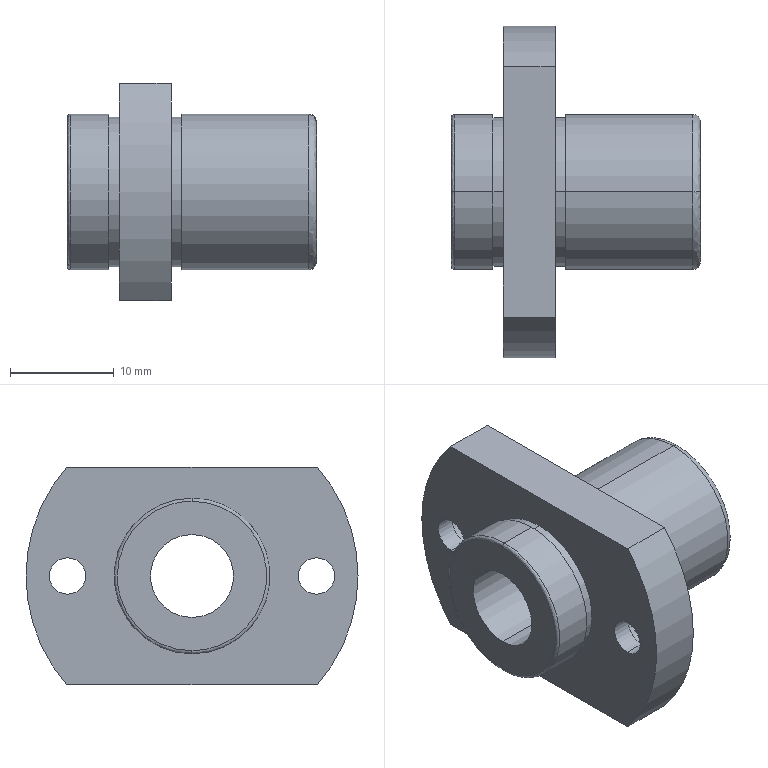Part | STEP file | LHIFC-N8 | 1 solid | 34 faces | box 24 x 32 x 21 mm | volume 5005 mm3 | cylinder 20 | plane 10 | spline 4 | commonest cylinder face diameters 3.5 x4 6 x4 14.4 x4 15 x4 8 x2 32 x2
STEP:
#1=CARTESIAN_POINT('',(0.,0.,7.2));
#2=VERTEX_POINT('',#1);
#3=CARTESIAN_POINT('',(0.,0.,-7.2));
#4=VERTEX_POINT('',#3);
#5=CARTESIAN_POINT('',(0.,0.,7.2));
#6=CARTESIAN_POINT('',(0.,-14.4,7.2));
#7=CARTESIAN_POINT('',(0.,-14.4,-7.2));
#8=CARTESIAN_POINT('',(0.,0.,-7.2));
#9=(BOUNDED_CURVE()B_SPLINE_CURVE(3,(#5,#6,#7,#8),.UNSPECIFIED.,.F.,.F.)B_SPLINE_CURVE_WITH_KNOTS((4,4),(0.,1.),.UNSPECIFIED.)CURVE()GEOMETRIC_REPRESENTATION_ITEM()RATIONAL_B_SPLINE_CURVE((1.,0.3333,0.3333,1.))REPRESENTATION_ITEM(''));
#10=EDGE_CURVE('',#2,#4,#9,.T.);
#11=ORIENTED_EDGE('',*,*,#10,.T.);
#12=CARTESIAN_POINT('',(0.3,0.,-7.5));
#13=VERTEX_POINT('',#12);
#14=CARTESIAN_POINT('',(0.3,0.,-7.2));
#15=DIRECTION('',(0.,-1.,0.));
#16=DIRECTION('',(0.,0.,-1.));
#17=AXIS2_PLACEMENT_3D('',#14,#15,#16);
#18=CIRCLE('',#17,0.3);
#19=EDGE_CURVE('',#4,#13,#18,.T.);
#20=ORIENTED_EDGE('',*,*,#19,.T.);
#21=CARTESIAN_POINT('',(0.3,0.,7.5));
#22=VERTEX_POINT('',#21);
#23=CARTESIAN_POINT('',(0.3,0.,0.));
#24=DIRECTION('',(1.,0.,0.));
#25=DIRECTION('',(0.,0.,-1.));
#26=AXIS2_PLACEMENT_3D('',#23,#24,#25);
#27=CIRCLE('',#26,7.5);
#28=EDGE_CURVE('',#22,#13,#27,.T.);
#29=ORIENTED_EDGE('',*,*,#28,.F.);
#30=CARTESIAN_POINT('',(0.3,0.,7.2));
#31=DIRECTION('',(0.,1.,0.));
#32=DIRECTION('',(0.,0.,1.));
#33=AXIS2_PLACEMENT_3D('',#30,#31,#32);
#34=CIRCLE('',#33,0.3);
#35=EDGE_CURVE('',#2,#22,#34,.T.);
#36=ORIENTED_EDGE('',*,*,#35,.F.);
#37=EDGE_LOOP('',(#11,#20,#29,#36));
#38=FACE_OUTER_BOUND('',#37,.T.);
#39=CARTESIAN_POINT('',(0.,0.,-7.2));
#40=CARTESIAN_POINT('',(0.,-14.4,-7.2));
#41=CARTESIAN_POINT('',(0.,-14.4,7.2));
#42=CARTESIAN_POINT('',(0.,0.,7.2));
#43=CARTESIAN_POINT('',(0.,0.,-7.376));
#44=CARTESIAN_POINT('',(0.,-14.751,-7.376));
#45=CARTESIAN_POINT('',(0.,-14.751,7.376));
#46=CARTESIAN_POINT('',(0.,0.,7.376));
#47=CARTESIAN_POINT('',(0.1243,0.,-7.5));
#48=CARTESIAN_POINT('',(0.1243,-15.,-7.5));
#49=CARTESIAN_POINT('',(0.1243,-15.,7.5));
#50=CARTESIAN_POINT('',(0.1243,0.,7.5));
#51=CARTESIAN_POINT('',(0.3,0.,-7.5));
#52=CARTESIAN_POINT('',(0.3,-15.,-7.5));
#53=CARTESIAN_POINT('',(0.3,-15.,7.5));
#54=CARTESIAN_POINT('',(0.3,0.,7.5));
#55=(BOUNDED_SURFACE()B_SPLINE_SURFACE(3,3,((#39,#40,#41,#42),(#43,#44,#45,#46),(#47,#48,#49,#50),(#51,#52,#53,#54)),.UNSPECIFIED.,.F.,.F.,.F.)B_SPLINE_SURFACE_WITH_KNOTS((4,4),(4,4),(0.,1.),(0.,1.),.UNSPECIFIED.)GEOMETRIC_REPRESENTATION_ITEM()RATIONAL_B_SPLINE_SURFACE(((1.,0.3333,0.3333,1.),(0.8047,0.2682,0.2682,0.8047),(0.8047,0.2682,0.2682,0.8047),(1.,0.3333,0.3333,1.)))REPRESENTATION_ITEM('')SURFACE());
#56=ADVANCED_FACE('',(#38),#55,.T.);
#57=CARTESIAN_POINT('',(23.25,0.,-7.5));
#58=VERTEX_POINT('',#57);
#59=CARTESIAN_POINT('',(23.25,0.,7.5));
#60=VERTEX_POINT('',#59);
#61=CARTESIAN_POINT('',(23.25,0.,0.));
#62=DIRECTION('',(-1.,0.,0.));
#63=DIRECTION('',(0.,0.,-1.));
#64=AXIS2_PLACEMENT_3D('',#61,#62,#63);
#65=CIRCLE('',#64,7.5);
#66=EDGE_CURVE('',#58,#60,#65,.T.);
#67=ORIENTED_EDGE('',*,*,#66,.F.);
#68=CARTESIAN_POINT('',(24.,0.,-6.75));
#69=VERTEX_POINT('',#68);
#70=CARTESIAN_POINT('',(23.25,0.,-6.75));
#71=DIRECTION('',(0.,-1.,0.));
#72=DIRECTION('',(0.,0.,-1.));
#73=AXIS2_PLACEMENT_3D('',#70,#71,#72);
#74=CIRCLE('',#73,0.75);
#75=EDGE_CURVE('',#58,#69,#74,.T.);
#76=ORIENTED_EDGE('',*,*,#75,.T.);
#77=CARTESIAN_POINT('',(24.,0.,6.75));
#78=VERTEX_POINT('',#77);
#79=CARTESIAN_POINT('',(24.,0.,-6.75));
#80=CARTESIAN_POINT('',(24.,-13.5,-6.75));
#81=CARTESIAN_POINT('',(24.,-13.5,6.75));
#82=CARTESIAN_POINT('',(24.,0.,6.75));
#83=(BOUNDED_CURVE()B_SPLINE_CURVE(3,(#79,#80,#81,#82),.UNSPECIFIED.,.F.,.F.)B_SPLINE_CURVE_WITH_KNOTS((4,4),(0.,1.),.UNSPECIFIED.)CURVE()GEOMETRIC_REPRESENTATION_ITEM()RATIONAL_B_SPLINE_CURVE((1.,0.3333,0.3333,1.))REPRESENTATION_ITEM(''));
#84=EDGE_CURVE('',#69,#78,#83,.T.);
#85=ORIENTED_EDGE('',*,*,#84,.T.);
#86=CARTESIAN_POINT('',(23.25,0.,6.75));
#87=DIRECTION('',(0.,1.,0.));
#88=DIRECTION('',(0.,0.,1.));
#89=AXIS2_PLACEMENT_3D('',#86,#87,#88);
#90=CIRCLE('',#89,0.75);
#91=EDGE_CURVE('',#60,#78,#90,.T.);
#92=ORIENTED_EDGE('',*,*,#91,.F.);
#93=EDGE_LOOP('',(#67,#76,#85,#92));
#94=FACE_OUTER_BOUND('',#93,.T.);
#95=CARTESIAN_POINT('',(23.25,0.,-7.5));
#96=CARTESIAN_POINT('',(23.25,-15.,-7.5));
#97=CARTESIAN_POINT('',(23.25,-15.,7.5));
#98=CARTESIAN_POINT('',(23.25,0.,7.5));
#99=CARTESIAN_POINT('',(23.689,0.,-7.5));
#100=CARTESIAN_POINT('',(23.689,-15.,-7.5));
#101=CARTESIAN_POINT('',(23.689,-15.,7.5));
#102=CARTESIAN_POINT('',(23.689,0.,7.5));
#103=CARTESIAN_POINT('',(24.,0.,-7.189));
#104=CARTESIAN_POINT('',(24.,-14.379,-7.189));
#105=CARTESIAN_POINT('',(24.,-14.379,7.189));
#106=CARTESIAN_POINT('',(24.,0.,7.189));
#107=CARTESIAN_POINT('',(24.,0.,-6.75));
#108=CARTESIAN_POINT('',(24.,-13.5,-6.75));
#109=CARTESIAN_POINT('',(24.,-13.5,6.75));
#110=CARTESIAN_POINT('',(24.,0.,6.75));
#111=(BOUNDED_SURFACE()B_SPLINE_SURFACE(3,3,((#95,#96,#97,#98),(#99,#100,#101,#102),(#103,#104,#105,#106),(#107,#108,#109,#110)),.UNSPECIFIED.,.F.,.F.,.F.)B_SPLINE_SURFACE_WITH_KNOTS((4,4),(4,4),(0.,1.),(0.,1.),.UNSPECIFIED.)GEOMETRIC_REPRESENTATION_ITEM()RATIONAL_B_SPLINE_SURFACE(((1.,0.3333,0.3333,1.),(0.8047,0.2682,0.2682,0.8047),(0.8047,0.2682,0.2682,0.8047),(1.,0.3333,0.3333,1.)))REPRESENTATION_ITEM('')SURFACE());
#112=ADVANCED_FACE('',(#94),#111,.T.);
#113=CARTESIAN_POINT('',(4.,0.,-7.2));
#114=VERTEX_POINT('',#113);
#115=CARTESIAN_POINT('',(4.,0.,7.2));
#116=VERTEX_POINT('',#115);
#117=CARTESIAN_POINT('',(4.,0.,0.));
#118=DIRECTION('',(1.,0.,0.));
#119=DIRECTION('',(0.,0.,-1.));
#120=AXIS2_PLACEMENT_3D('',#117,#118,#119);
#121=CIRCLE('',#120,7.2);
#122=EDGE_CURVE('',#114,#116,#121,.T.);
#123=ORIENTED_EDGE('',*,*,#122,.T.);
#124=CARTESIAN_POINT('',(5.,0.,7.2));
#125=VERTEX_POINT('',#124);
#126=CARTESIAN_POINT('',(4.5,0.,7.2));
#127=DIRECTION('',(1.,0.,0.));
#128=VECTOR('',#127,1000.);
#129=LINE('',#126,#128);
#130=EDGE_CURVE('',#116,#125,#129,.T.);
#131=ORIENTED_EDGE('',*,*,#130,.T.);
#132=CARTESIAN_POINT('',(5.,0.,-7.2));
#133=VERTEX_POINT('',#132);
#134=CARTESIAN_POINT('',(5.,0.,0.));
#135=DIRECTION('',(1.,0.,0.));
#136=DIRECTION('',(0.,0.,-1.));
#137=AXIS2_PLACEMENT_3D('',#134,#135,#136);
#138=CIRCLE('',#137,7.2);
#139=EDGE_CURVE('',#133,#125,#138,.T.);
#140=ORIENTED_EDGE('',*,*,#139,.F.);
#141=CARTESIAN_POINT('',(4.5,0.,-7.2));
#142=DIRECTION('',(1.,0.,0.));
#143=VECTOR('',#142,1000.);
#144=LINE('',#141,#143);
#145=EDGE_CURVE('',#114,#133,#144,.T.);
#146=ORIENTED_EDGE('',*,*,#145,.F.);
#147=EDGE_LOOP('',(#123,#131,#140,#146));
#148=FACE_OUTER_BOUND('',#147,.T.);
#149=CARTESIAN_POINT('',(4.5,0.,0.));
#150=DIRECTION('',(1.,0.,0.));
#151=DIRECTION('',(0.,0.,-1.));
#152=AXIS2_PLACEMENT_3D('',#149,#150,#151);
#153=CYLINDRICAL_SURFACE('',#152,7.2);
#154=ADVANCED_FACE('',(#148),#153,.T.);
#155=CARTESIAN_POINT('',(5.,12.,1.75));
#156=VERTEX_POINT('',#155);
#157=CARTESIAN_POINT('',(5.,12.,-1.75));
#158=VERTEX_POINT('',#157);
#159=CARTESIAN_POINT('',(5.,12.,0.));
#160=DIRECTION('',(1.,0.,0.));
#161=DIRECTION('',(0.,0.,-1.));
#162=AXIS2_PLACEMENT_3D('',#159,#160,#161);
#163=CIRCLE('',#162,1.75);
#164=EDGE_CURVE('',#156,#158,#163,.T.);
#165=ORIENTED_EDGE('',*,*,#164,.F.);
#166=CARTESIAN_POINT('',(6.9,12.,1.75));
#167=VERTEX_POINT('',#166);
#168=CARTESIAN_POINT('',(5.95,12.,1.75));
#169=DIRECTION('',(1.,0.,0.));
#170=VECTOR('',#169,1000.);
#171=LINE('',#168,#170);
#172=EDGE_CURVE('',#156,#167,#171,.T.);
#173=ORIENTED_EDGE('',*,*,#172,.T.);
#174=CARTESIAN_POINT('',(6.9,12.,-1.75));
#175=VERTEX_POINT('',#174);
#176=CARTESIAN_POINT('',(6.9,12.,0.));
#177=DIRECTION('',(-1.,0.,0.));
#178=DIRECTION('',(0.,0.,-1.));
#179=AXIS2_PLACEMENT_3D('',#176,#177,#178);
#180=CIRCLE('',#179,1.75);
#181=EDGE_CURVE('',#175,#167,#180,.T.);
#182=ORIENTED_EDGE('',*,*,#181,.F.);
#183=CARTESIAN_POINT('',(5.95,12.,-1.75));
#184=DIRECTION('',(1.,0.,0.));
#185=VECTOR('',#184,1000.);
#186=LINE('',#183,#185);
#187=EDGE_CURVE('',#158,#175,#186,.T.);
#188=ORIENTED_EDGE('',*,*,#187,.F.);
#189=EDGE_LOOP('',(#165,#173,#182,#188));
#190=FACE_OUTER_BOUND('',#189,.T.);
#191=CARTESIAN_POINT('',(5.95,12.,0.));
#192=DIRECTION('',(1.,0.,0.));
#193=DIRECTION('',(0.,0.,-1.));
#194=AXIS2_PLACEMENT_3D('',#191,#192,#193);
#195=CYLINDRICAL_SURFACE('',#194,1.75);
#196=ADVANCED_FACE('',(#190),#195,.F.);
#197=CARTESIAN_POINT('',(5.,-12.,1.75));
#198=VERTEX_POINT('',#197);
#199=CARTESIAN_POINT('',(5.,-12.,-1.75));
#200=VERTEX_POINT('',#199);
#201=CARTESIAN_POINT('',(5.,-12.,0.));
#202=DIRECTION('',(1.,0.,0.));
#203=DIRECTION('',(0.,0.,-1.));
#204=AXIS2_PLACEMENT_3D('',#201,#202,#203);
#205=CIRCLE('',#204,1.75);
#206=EDGE_CURVE('',#198,#200,#205,.T.);
#207=ORIENTED_EDGE('',*,*,#206,.F.);
#208=CARTESIAN_POINT('',(6.9,-12.,1.75));
#209=VERTEX_POINT('',#208);
#210=CARTESIAN_POINT('',(5.95,-12.,1.75));
#211=DIRECTION('',(1.,0.,0.));
#212=VECTOR('',#211,1000.);
#213=LINE('',#210,#212);
#214=EDGE_CURVE('',#198,#209,#213,.T.);
#215=ORIENTED_EDGE('',*,*,#214,.T.);
#216=CARTESIAN_POINT('',(6.9,-12.,-1.75));
#217=VERTEX_POINT('',#216);
#218=CARTESIAN_POINT('',(6.9,-12.,0.));
#219=DIRECTION('',(-1.,0.,0.));
#220=DIRECTION('',(0.,0.,-1.));
#221=AXIS2_PLACEMENT_3D('',#218,#219,#220);
#222=CIRCLE('',#221,1.75);
#223=EDGE_CURVE('',#217,#209,#222,.T.);
#224=ORIENTED_EDGE('',*,*,#223,.F.);
#225=CARTESIAN_POINT('',(5.95,-12.,-1.75));
#226=DIRECTION('',(1.,0.,0.));
#227=VECTOR('',#226,1000.);
#228=LINE('',#225,#227);
#229=EDGE_CURVE('',#200,#217,#228,.T.);
#230=ORIENTED_EDGE('',*,*,#229,.F.);
#231=EDGE_LOOP('',(#207,#215,#224,#230));
#232=FACE_OUTER_BOUND('',#231,.T.);
#233=CARTESIAN_POINT('',(5.95,-12.,0.));
#234=DIRECTION('',(1.,0.,0.));
#235=DIRECTION('',(0.,0.,-1.));
#236=AXIS2_PLACEMENT_3D('',#233,#234,#235);
#237=CYLINDRICAL_SURFACE('',#236,1.75);
#238=ADVANCED_FACE('',(#232),#237,.F.);
#239=CARTESIAN_POINT('',(0.3,0.,0.));
#240=DIRECTION('',(1.,0.,0.));
#241=DIRECTION('',(0.,0.,-1.));
#242=AXIS2_PLACEMENT_3D('',#239,#240,#241);
#243=CIRCLE('',#242,7.5);
#244=EDGE_CURVE('',#13,#22,#243,.T.);
#245=ORIENTED_EDGE('',*,*,#244,.T.);
#246=CARTESIAN_POINT('',(4.,0.,7.5));
#247=VERTEX_POINT('',#246);
#248=CARTESIAN_POINT('',(2.15,0.,7.5));
#249=DIRECTION('',(1.,0.,0.));
#250=VECTOR('',#249,1000.);
#251=LINE('',#248,#250);
#252=EDGE_CURVE('',#22,#247,#251,.T.);
#253=ORIENTED_EDGE('',*,*,#252,.T.);
#254=CARTESIAN_POINT('',(4.,0.,-7.5));
#255=VERTEX_POINT('',#254);
#256=CARTESIAN_POINT('',(4.,0.,0.));
#257=DIRECTION('',(1.,0.,0.));
#258=DIRECTION('',(0.,0.,-1.));
#259=AXIS2_PLACEMENT_3D('',#256,#257,#258);
#260=CIRCLE('',#259,7.5);
#261=EDGE_CURVE('',#255,#247,#260,.T.);
#262=ORIENTED_EDGE('',*,*,#261,.F.);
#263=CARTESIAN_POINT('',(2.15,0.,-7.5));
#264=DIRECTION('',(1.,0.,0.));
#265=VECTOR('',#264,1000.);
#266=LINE('',#263,#265);
#267=EDGE_CURVE('',#13,#255,#266,.T.);
#268=ORIENTED_EDGE('',*,*,#267,.F.);
#269=EDGE_LOOP('',(#245,#253,#262,#268));
#270=FACE_OUTER_BOUND('',#269,.T.);
#271=CARTESIAN_POINT('',(2.15,0.,0.));
#272=DIRECTION('',(1.,0.,0.));
#273=DIRECTION('',(0.,0.,-1.));
#274=AXIS2_PLACEMENT_3D('',#271,#272,#273);
#275=CYLINDRICAL_SURFACE('',#274,7.5);
#276=ADVANCED_FACE('',(#270),#275,.T.);
#277=CARTESIAN_POINT('',(10.,0.,7.2));
#278=VERTEX_POINT('',#277);
#279=CARTESIAN_POINT('',(10.,0.,-7.2));
#280=VERTEX_POINT('',#279);
#281=CARTESIAN_POINT('',(10.,0.,0.));
#282=DIRECTION('',(-1.,0.,0.));
#283=DIRECTION('',(0.,0.,-1.));
#284=AXIS2_PLACEMENT_3D('',#281,#282,#283);
#285=CIRCLE('',#284,7.2);
#286=EDGE_CURVE('',#278,#280,#285,.T.);
#287=ORIENTED_EDGE('',*,*,#286,.F.);
#288=CARTESIAN_POINT('',(11.,0.,7.2));
#289=VERTEX_POINT('',#288);
#290=CARTESIAN_POINT('',(10.5,0.,7.2));
#291=DIRECTION('',(1.,0.,0.));
#292=VECTOR('',#291,1000.);
#293=LINE('',#290,#292);
#294=EDGE_CURVE('',#278,#289,#293,.T.);
#295=ORIENTED_EDGE('',*,*,#294,.T.);
#296=CARTESIAN_POINT('',(11.,0.,-7.2));
#297=VERTEX_POINT('',#296);
#298=CARTESIAN_POINT('',(11.,0.,0.));
#299=DIRECTION('',(-1.,0.,0.));
#300=DIRECTION('',(0.,0.,-1.));
#301=AXIS2_PLACEMENT_3D('',#298,#299,#300);
#302=CIRCLE('',#301,7.2);
#303=EDGE_CURVE('',#289,#297,#302,.T.);
#304=ORIENTED_EDGE('',*,*,#303,.T.);
#305=CARTESIAN_POINT('',(10.5,0.,-7.2));
#306=DIRECTION('',(1.,0.,0.));
#307=VECTOR('',#306,1000.);
#308=LINE('',#305,#307);
#309=EDGE_CURVE('',#280,#297,#308,.T.);
#310=ORIENTED_EDGE('',*,*,#309,.F.);
#311=EDGE_LOOP('',(#287,#295,#304,#310));
#312=FACE_OUTER_BOUND('',#311,.T.);
#313=CARTESIAN_POINT('',(10.5,0.,0.));
#314=DIRECTION('',(1.,0.,0.));
#315=DIRECTION('',(0.,0.,-1.));
#316=AXIS2_PLACEMENT_3D('',#313,#314,#315);
#317=CYLINDRICAL_SURFACE('',#316,7.2);
#318=ADVANCED_FACE('',(#312),#317,.T.);
#319=CARTESIAN_POINT('',(6.9,12.,-3.));
#320=VERTEX_POINT('',#319);
#321=CARTESIAN_POINT('',(6.9,12.,3.));
#322=VERTEX_POINT('',#321);
#323=CARTESIAN_POINT('',(6.9,12.,0.));
#324=DIRECTION('',(-1.,0.,0.));
#325=DIRECTION('',(0.,0.,-1.));
#326=AXIS2_PLACEMENT_3D('',#323,#324,#325);
#327=CIRCLE('',#326,3.);
#328=EDGE_CURVE('',#320,#322,#327,.T.);
#329=ORIENTED_EDGE('',*,*,#328,.T.);
#330=CARTESIAN_POINT('',(10.,12.,3.));
#331=VERTEX_POINT('',#330);
#332=CARTESIAN_POINT('',(8.45,12.,3.));
#333=DIRECTION('',(1.,0.,0.));
#334=VECTOR('',#333,1000.);
#335=LINE('',#332,#334);
#336=EDGE_CURVE('',#322,#331,#335,.T.);
#337=ORIENTED_EDGE('',*,*,#336,.T.);
#338=CARTESIAN_POINT('',(10.,12.,-3.));
#339=VERTEX_POINT('',#338);
#340=CARTESIAN_POINT('',(10.,12.,0.));
#341=DIRECTION('',(-1.,0.,0.));
#342=DIRECTION('',(0.,0.,-1.));
#343=AXIS2_PLACEMENT_3D('',#340,#341,#342);
#344=CIRCLE('',#343,3.);
#345=EDGE_CURVE('',#339,#331,#344,.T.);
#346=ORIENTED_EDGE('',*,*,#345,.F.);
#347=CARTESIAN_POINT('',(8.45,12.,-3.));
#348=DIRECTION('',(1.,0.,0.));
#349=VECTOR('',#348,1000.);
#350=LINE('',#347,#349);
#351=EDGE_CURVE('',#320,#339,#350,.T.);
#352=ORIENTED_EDGE('',*,*,#351,.F.);
#353=EDGE_LOOP('',(#329,#337,#346,#352));
#354=FACE_OUTER_BOUND('',#353,.T.);
#355=CARTESIAN_POINT('',(8.45,12.,0.));
#356=DIRECTION('',(1.,0.,0.));
#357=DIRECTION('',(0.,0.,-1.));
#358=AXIS2_PLACEMENT_3D('',#355,#356,#357);
#359=CYLINDRICAL_SURFACE('',#358,3.);
#360=ADVANCED_FACE('',(#354),#359,.F.);
#361=CARTESIAN_POINT('',(6.9,-12.,-3.));
#362=VERTEX_POINT('',#361);
#363=CARTESIAN_POINT('',(6.9,-12.,3.));
#364=VERTEX_POINT('',#363);
#365=CARTESIAN_POINT('',(6.9,-12.,0.));
#366=DIRECTION('',(-1.,0.,0.));
#367=DIRECTION('',(0.,0.,-1.));
#368=AXIS2_PLACEMENT_3D('',#365,#366,#367);
#369=CIRCLE('',#368,3.);
#370=EDGE_CURVE('',#362,#364,#369,.T.);
#371=ORIENTED_EDGE('',*,*,#370,.T.);
#372=CARTESIAN_POINT('',(10.,-12.,3.));
#373=VERTEX_POINT('',#372);
#374=CARTESIAN_POINT('',(8.45,-12.,3.));
#375=DIRECTION('',(1.,0.,0.));
#376=VECTOR('',#375,1000.);
#377=LINE('',#374,#376);
#378=EDGE_CURVE('',#364,#373,#377,.T.);
#379=ORIENTED_EDGE('',*,*,#378,.T.);
#380=CARTESIAN_POINT('',(10.,-12.,-3.));
#381=VERTEX_POINT('',#380);
#382=CARTESIAN_POINT('',(10.,-12.,0.));
#383=DIRECTION('',(-1.,0.,0.));
#384=DIRECTION('',(0.,0.,-1.));
#385=AXIS2_PLACEMENT_3D('',#382,#383,#384);
#386=CIRCLE('',#385,3.);
#387=EDGE_CURVE('',#381,#373,#386,.T.);
#388=ORIENTED_EDGE('',*,*,#387,.F.);
#389=CARTESIAN_POINT('',(8.45,-12.,-3.));
#390=DIRECTION('',(1.,0.,0.));
#391=VECTOR('',#390,1000.);
#392=LINE('',#389,#391);
#393=EDGE_CURVE('',#362,#381,#392,.T.);
#394=ORIENTED_EDGE('',*,*,#393,.F.);
#395=EDGE_LOOP('',(#371,#379,#388,#394));
#396=FACE_OUTER_BOUND('',#395,.T.);
#397=CARTESIAN_POINT('',(8.45,-12.,0.));
#398=DIRECTION('',(1.,0.,0.));
#399=DIRECTION('',(0.,0.,-1.));
#400=AXIS2_PLACEMENT_3D('',#397,#398,#399);
#401=CYLINDRICAL_SURFACE('',#400,3.);
#402=ADVANCED_FACE('',(#396),#401,.F.);
#403=CARTESIAN_POINT('',(11.,0.,7.5));
#404=VERTEX_POINT('',#403);
#405=CARTESIAN_POINT('',(11.,0.,-7.5));
#406=VERTEX_POINT('',#405);
#407=CARTESIAN_POINT('',(11.,0.,0.));
#408=DIRECTION('',(-1.,0.,0.));
#409=DIRECTION('',(0.,0.,-1.));
#410=AXIS2_PLACEMENT_3D('',#407,#408,#409);
#411=CIRCLE('',#410,7.5);
#412=EDGE_CURVE('',#404,#406,#411,.T.);
#413=ORIENTED_EDGE('',*,*,#412,.F.);
#414=CARTESIAN_POINT('',(17.125,0.,7.5));
#415=DIRECTION('',(1.,0.,0.));
#416=VECTOR('',#415,1000.);
#417=LINE('',#414,#416);
#418=EDGE_CURVE('',#404,#60,#417,.T.);
#419=ORIENTED_EDGE('',*,*,#418,.T.);
#420=CARTESIAN_POINT('',(23.25,0.,0.));
#421=DIRECTION('',(-1.,0.,0.));
#422=DIRECTION('',(0.,0.,-1.));
#423=AXIS2_PLACEMENT_3D('',#420,#421,#422);
#424=CIRCLE('',#423,7.5);
#425=EDGE_CURVE('',#60,#58,#424,.T.);
#426=ORIENTED_EDGE('',*,*,#425,.T.);
#427=CARTESIAN_POINT('',(17.125,0.,-7.5));
#428=DIRECTION('',(1.,0.,0.));
#429=VECTOR('',#428,1000.);
#430=LINE('',#427,#429);
#431=EDGE_CURVE('',#406,#58,#430,.T.);
#432=ORIENTED_EDGE('',*,*,#431,.F.);
#433=EDGE_LOOP('',(#413,#419,#426,#432));
#434=FACE_OUTER_BOUND('',#433,.T.);
#435=CARTESIAN_POINT('',(17.125,0.,0.));
#436=DIRECTION('',(1.,0.,0.));
#437=DIRECTION('',(0.,0.,-1.));
#438=AXIS2_PLACEMENT_3D('',#435,#436,#437);
#439=CYLINDRICAL_SURFACE('',#438,7.5);
#440=ADVANCED_FACE('',(#434),#439,.T.);
#441=CARTESIAN_POINT('',(0.,0.,4.));
#442=VERTEX_POINT('',#441);
#443=CARTESIAN_POINT('',(0.,0.,-4.));
#444=VERTEX_POINT('',#443);
#445=CARTESIAN_POINT('',(0.,0.,0.));
#446=DIRECTION('',(1.,0.,0.));
#447=DIRECTION('',(0.,0.,-1.));
#448=AXIS2_PLACEMENT_3D('',#445,#446,#447);
#449=CIRCLE('',#448,4.);
#450=EDGE_CURVE('',#442,#444,#449,.T.);
#451=ORIENTED_EDGE('',*,*,#450,.F.);
#452=CARTESIAN_POINT('',(24.,0.,4.));
#453=VERTEX_POINT('',#452);
#454=CARTESIAN_POINT('',(12.,0.,4.));
#455=DIRECTION('',(1.,0.,0.));
#456=VECTOR('',#455,1000.);
#457=LINE('',#454,#456);
#458=EDGE_CURVE('',#442,#453,#457,.T.);
#459=ORIENTED_EDGE('',*,*,#458,.T.);
#460=CARTESIAN_POINT('',(24.,0.,-4.));
#461=VERTEX_POINT('',#460);
#462=CARTESIAN_POINT('',(24.,0.,0.));
#463=DIRECTION('',(-1.,0.,0.));
#464=DIRECTION('',(0.,0.,-1.));
#465=AXIS2_PLACEMENT_3D('',#462,#463,#464);
#466=CIRCLE('',#465,4.);
#467=EDGE_CURVE('',#461,#453,#466,.T.);
#468=ORIENTED_EDGE('',*,*,#467,.F.);
#469=CARTESIAN_POINT('',(12.,0.,-4.));
#470=DIRECTION('',(1.,0.,0.));
#471=VECTOR('',#470,1000.);
#472=LINE('',#469,#471);
#473=EDGE_CURVE('',#444,#461,#472,.T.);
#474=ORIENTED_EDGE('',*,*,#473,.F.);
#475=EDGE_LOOP('',(#451,#459,#468,#474));
#476=FACE_OUTER_BOUND('',#475,.T.);
#477=CARTESIAN_POINT('',(12.,0.,0.));
#478=DIRECTION('',(1.,0.,0.));
#479=DIRECTION('',(0.,0.,-1.));
#480=AXIS2_PLACEMENT_3D('',#477,#478,#479);
#481=CYLINDRICAL_SURFACE('',#480,4.);
#482=ADVANCED_FACE('',(#476),#481,.F.);
#483=ORIENTED_EDGE('',*,*,#139,.T.);
#484=CARTESIAN_POINT('',(5.,0.,0.));
#485=DIRECTION('',(1.,0.,0.));
#486=DIRECTION('',(0.,0.,-1.));
#487=AXIS2_PLACEMENT_3D('',#484,#485,#486);
#488=CIRCLE('',#487,7.2);
#489=EDGE_CURVE('',#125,#133,#488,.T.);
#490=ORIENTED_EDGE('',*,*,#489,.T.);
#491=EDGE_LOOP('',(#483,#490));
#492=FACE_BOUND('',#491,.T.);
#493=CARTESIAN_POINT('',(5.,12.073,10.5));
#494=VERTEX_POINT('',#493);
#495=CARTESIAN_POINT('',(5.,12.073,-10.5));
#496=VERTEX_POINT('',#495);
#497=CARTESIAN_POINT('',(5.,0.,0.));
#498=DIRECTION('',(-1.,0.,0.));
#499=DIRECTION('',(0.,0.,-1.));
#500=AXIS2_PLACEMENT_3D('',#497,#498,#499);
#501=CIRCLE('',#500,16.);
#502=EDGE_CURVE('',#494,#496,#501,.T.);
#503=ORIENTED_EDGE('',*,*,#502,.T.);
#504=CARTESIAN_POINT('',(5.,-12.073,-10.5));
#505=VERTEX_POINT('',#504);
#506=CARTESIAN_POINT('',(5.,11.6,-10.5));
#507=DIRECTION('',(0.,-1.,0.));
#508=VECTOR('',#507,1000.);
#509=LINE('',#506,#508);
#510=EDGE_CURVE('',#496,#505,#509,.T.);
#511=ORIENTED_EDGE('',*,*,#510,.T.);
#512=CARTESIAN_POINT('',(5.,-12.073,10.5));
#513=VERTEX_POINT('',#512);
#514=CARTESIAN_POINT('',(5.,0.,0.));
#515=DIRECTION('',(-1.,0.,0.));
#516=DIRECTION('',(0.,0.,-1.));
#517=AXIS2_PLACEMENT_3D('',#514,#515,#516);
#518=CIRCLE('',#517,16.);
#519=EDGE_CURVE('',#505,#513,#518,.T.);
#520=ORIENTED_EDGE('',*,*,#519,.T.);
#521=CARTESIAN_POINT('',(5.,11.6,10.5));
#522=DIRECTION('',(0.,1.,0.));
#523=VECTOR('',#522,1000.);
#524=LINE('',#521,#523);
#525=EDGE_CURVE('',#513,#494,#524,.T.);
#526=ORIENTED_EDGE('',*,*,#525,.T.);
#527=EDGE_LOOP('',(#503,#511,#520,#526));
#528=FACE_OUTER_BOUND('',#527,.T.);
#529=CARTESIAN_POINT('',(5.,12.,0.));
#530=DIRECTION('',(1.,0.,0.));
#531=DIRECTION('',(0.,0.,-1.));
#532=AXIS2_PLACEMENT_3D('',#529,#530,#531);
#533=CIRCLE('',#532,1.75);
#534=EDGE_CURVE('',#158,#156,#533,.T.);
#535=ORIENTED_EDGE('',*,*,#534,.T.);
#536=ORIENTED_EDGE('',*,*,#164,.T.);
#537=EDGE_LOOP('',(#535,#536));
#538=FACE_BOUND('',#537,.T.);
#539=CARTESIAN_POINT('',(5.,-12.,0.));
#540=DIRECTION('',(1.,0.,0.));
#541=DIRECTION('',(0.,0.,-1.));
#542=AXIS2_PLACEMENT_3D('',#539,#540,#541);
#543=CIRCLE('',#542,1.75);
#544=EDGE_CURVE('',#200,#198,#543,.T.);
#545=ORIENTED_EDGE('',*,*,#544,.T.);
#546=ORIENTED_EDGE('',*,*,#206,.T.);
#547=EDGE_LOOP('',(#545,#546));
#548=FACE_BOUND('',#547,.T.);
#549=CARTESIAN_POINT('',(5.,11.6,0.));
#550=DIRECTION('',(-1.,0.,0.));
#551=DIRECTION('',(0.,0.,1.));
#552=AXIS2_PLACEMENT_3D('',#549,#550,#551);
#553=PLANE('',#552);
#554=ADVANCED_FACE('',(#492,#528,#538,#548),#553,.T.);
#555=ORIENTED_EDGE('',*,*,#130,.F.);
#556=CARTESIAN_POINT('',(4.,0.,0.));
#557=DIRECTION('',(1.,0.,0.));
#558=DIRECTION('',(0.,0.,-1.));
#559=AXIS2_PLACEMENT_3D('',#556,#557,#558);
#560=CIRCLE('',#559,7.2);
#561=EDGE_CURVE('',#116,#114,#560,.T.);
#562=ORIENTED_EDGE('',*,*,#561,.T.);
#563=ORIENTED_EDGE('',*,*,#145,.T.);
#564=ORIENTED_EDGE('',*,*,#489,.F.);
#565=EDGE_LOOP('',(#555,#562,#563,#564));
#566=FACE_OUTER_BOUND('',#565,.T.);
#567=CARTESIAN_POINT('',(4.5,0.,0.));
#568=DIRECTION('',(1.,0.,0.));
#569=DIRECTION('',(0.,0.,-1.));
#570=AXIS2_PLACEMENT_3D('',#567,#568,#569);
#571=CYLINDRICAL_SURFACE('',#570,7.2);
#572=ADVANCED_FACE('',(#566),#571,.T.);
#573=CARTESIAN_POINT('',(10.,12.073,-10.5));
#574=VERTEX_POINT('',#573);
#575=CARTESIAN_POINT('',(7.5,12.073,-10.5));
#576=DIRECTION('',(-1.,0.,0.));
#577=VECTOR('',#576,1000.);
#578=LINE('',#575,#577);
#579=EDGE_CURVE('',#574,#496,#578,.T.);
#580=ORIENTED_EDGE('',*,*,#579,.T.);
#581=ORIENTED_EDGE('',*,*,#502,.F.);
#582=CARTESIAN_POINT('',(10.,12.073,10.5));
#583=VERTEX_POINT('',#582);
#584=CARTESIAN_POINT('',(7.5,12.073,10.5));
#585=DIRECTION('',(1.,0.,0.));
#586=VECTOR('',#585,1000.);
#587=LINE('',#584,#586);
#588=EDGE_CURVE('',#494,#583,#587,.T.);
#589=ORIENTED_EDGE('',*,*,#588,.T.);
#590=CARTESIAN_POINT('',(10.,0.,0.));
#591=DIRECTION('',(-1.,0.,0.));
#592=DIRECTION('',(0.,0.,-1.));
#593=AXIS2_PLACEMENT_3D('',#590,#591,#592);
#594=CIRCLE('',#593,16.);
#595=EDGE_CURVE('',#583,#574,#594,.T.);
#596=ORIENTED_EDGE('',*,*,#595,.T.);
#597=EDGE_LOOP('',(#580,#581,#589,#596));
#598=FACE_OUTER_BOUND('',#597,.T.);
#599=CARTESIAN_POINT('',(7.5,0.,0.));
#600=DIRECTION('',(1.,0.,0.));
#601=DIRECTION('',(0.,0.,-1.));
#602=AXIS2_PLACEMENT_3D('',#599,#600,#601);
#603=CYLINDRICAL_SURFACE('',#602,16.);
#604=ADVANCED_FACE('',(#598),#603,.T.);
#605=CARTESIAN_POINT('',(10.,-12.073,10.5));
#606=VERTEX_POINT('',#605);
#607=CARTESIAN_POINT('',(0.,-12.073,10.5));
#608=DIRECTION('',(-1.,0.,0.));
#609=VECTOR('',#608,1000.);
#610=LINE('',#607,#609);
#611=EDGE_CURVE('',#606,#513,#610,.T.);
#612=ORIENTED_EDGE('',*,*,#611,.F.);
#613=CARTESIAN_POINT('',(10.,12.073,10.5));
#614=DIRECTION('',(0.,-1.,0.));
#615=VECTOR('',#614,1000.);
#616=LINE('',#613,#615);
#617=EDGE_CURVE('',#583,#606,#616,.T.);
#618=ORIENTED_EDGE('',*,*,#617,.F.);
#619=ORIENTED_EDGE('',*,*,#588,.F.);
#620=ORIENTED_EDGE('',*,*,#525,.F.);
#621=EDGE_LOOP('',(#612,#618,#619,#620));
#622=FACE_OUTER_BOUND('',#621,.T.);
#623=CARTESIAN_POINT('',(0.,12.073,10.5));
#624=DIRECTION('',(0.,0.,-1.));
#625=DIRECTION('',(-1.,0.,0.));
#626=AXIS2_PLACEMENT_3D('',#623,#624,#625);
#627=PLANE('',#626);
#628=ADVANCED_FACE('',(#622),#627,.F.);
#629=ORIENTED_EDGE('',*,*,#611,.T.);
#630=ORIENTED_EDGE('',*,*,#519,.F.);
#631=CARTESIAN_POINT('',(10.,-12.073,-10.5));
#632=VERTEX_POINT('',#631);
#633=CARTESIAN_POINT('',(7.5,-12.073,-10.5));
#634=DIRECTION('',(1.,0.,0.));
#635=VECTOR('',#634,1000.);
#636=LINE('',#633,#635);
#637=EDGE_CURVE('',#505,#632,#636,.T.);
#638=ORIENTED_EDGE('',*,*,#637,.T.);
#639=CARTESIAN_POINT('',(10.,0.,0.));
#640=DIRECTION('',(-1.,0.,0.));
#641=DIRECTION('',(0.,0.,-1.));
#642=AXIS2_PLACEMENT_3D('',#639,#640,#641);
#643=CIRCLE('',#642,16.);
#644=EDGE_CURVE('',#632,#606,#643,.T.);
#645=ORIENTED_EDGE('',*,*,#644,.T.);
#646=EDGE_LOOP('',(#629,#630,#638,#645));
#647=FACE_OUTER_BOUND('',#646,.T.);
#648=CARTESIAN_POINT('',(7.5,0.,0.));
#649=DIRECTION('',(1.,0.,0.));
#650=DIRECTION('',(0.,0.,-1.));
#651=AXIS2_PLACEMENT_3D('',#648,#649,#650);
#652=CYLINDRICAL_SURFACE('',#651,16.);
#653=ADVANCED_FACE('',(#647),#652,.T.);
#654=ORIENTED_EDGE('',*,*,#579,.F.);
#655=CARTESIAN_POINT('',(10.,-12.073,-10.5));
#656=DIRECTION('',(0.,1.,0.));
#657=VECTOR('',#656,1000.);
#658=LINE('',#655,#657);
#659=EDGE_CURVE('',#632,#574,#658,.T.);
#660=ORIENTED_EDGE('',*,*,#659,.F.);
#661=ORIENTED_EDGE('',*,*,#637,.F.);
#662=ORIENTED_EDGE('',*,*,#510,.F.);
#663=EDGE_LOOP('',(#654,#660,#661,#662));
#664=FACE_OUTER_BOUND('',#663,.T.);
#665=CARTESIAN_POINT('',(0.,-12.073,-10.5));
#666=DIRECTION('',(0.,0.,1.));
#667=DIRECTION('',(1.,0.,0.));
#668=AXIS2_PLACEMENT_3D('',#665,#666,#667);
#669=PLANE('',#668);
#670=ADVANCED_FACE('',(#664),#669,.F.);
#671=ORIENTED_EDGE('',*,*,#172,.F.);
#672=ORIENTED_EDGE('',*,*,#534,.F.);
#673=ORIENTED_EDGE('',*,*,#187,.T.);
#674=CARTESIAN_POINT('',(6.9,12.,0.));
#675=DIRECTION('',(-1.,0.,0.));
#676=DIRECTION('',(0.,0.,-1.));
#677=AXIS2_PLACEMENT_3D('',#674,#675,#676);
#678=CIRCLE('',#677,1.75);
#679=EDGE_CURVE('',#167,#175,#678,.T.);
#680=ORIENTED_EDGE('',*,*,#679,.F.);
#681=EDGE_LOOP('',(#671,#672,#673,#680));
#682=FACE_OUTER_BOUND('',#681,.T.);
#683=CARTESIAN_POINT('',(5.95,12.,0.));
#684=DIRECTION('',(1.,0.,0.));
#685=DIRECTION('',(0.,0.,-1.));
#686=AXIS2_PLACEMENT_3D('',#683,#684,#685);
#687=CYLINDRICAL_SURFACE('',#686,1.75);
#688=ADVANCED_FACE('',(#682),#687,.F.);
#689=ORIENTED_EDGE('',*,*,#214,.F.);
#690=ORIENTED_EDGE('',*,*,#544,.F.);
#691=ORIENTED_EDGE('',*,*,#229,.T.);
#692=CARTESIAN_POINT('',(6.9,-12.,0.));
#693=DIRECTION('',(-1.,0.,0.));
#694=DIRECTION('',(0.,0.,-1.));
#695=AXIS2_PLACEMENT_3D('',#692,#693,#694);
#696=CIRCLE('',#695,1.75);
#697=EDGE_CURVE('',#209,#217,#696,.T.);
#698=ORIENTED_EDGE('',*,*,#697,.F.);
#699=EDGE_LOOP('',(#689,#690,#691,#698));
#700=FACE_OUTER_BOUND('',#699,.T.);
#701=CARTESIAN_POINT('',(5.95,-12.,0.));
#702=DIRECTION('',(1.,0.,0.));
#703=DIRECTION('',(0.,0.,-1.));
#704=AXIS2_PLACEMENT_3D('',#701,#702,#703);
#705=CYLINDRICAL_SURFACE('',#704,1.75);
#706=ADVANCED_FACE('',(#700),#705,.F.);
#707=ORIENTED_EDGE('',*,*,#122,.F.);
#708=ORIENTED_EDGE('',*,*,#561,.F.);
#709=EDGE_LOOP('',(#707,#708));
#710=FACE_BOUND('',#709,.T.);
#711=ORIENTED_EDGE('',*,*,#261,.T.);
#712=CARTESIAN_POINT('',(4.,0.,0.));
#713=DIRECTION('',(1.,0.,0.));
#714=DIRECTION('',(0.,0.,-1.));
#715=AXIS2_PLACEMENT_3D('',#712,#713,#714);
#716=CIRCLE('',#715,7.5);
#717=EDGE_CURVE('',#247,#255,#716,.T.);
#718=ORIENTED_EDGE('',*,*,#717,.T.);
#719=EDGE_LOOP('',(#711,#718));
#720=FACE_OUTER_BOUND('',#719,.T.);
#721=CARTESIAN_POINT('',(4.,7.35,0.));
#722=DIRECTION('',(1.,0.,0.));
#723=DIRECTION('',(0.,0.,-1.));
#724=AXIS2_PLACEMENT_3D('',#721,#722,#723);
#725=PLANE('',#724);
#726=ADVANCED_FACE('',(#710,#720),#725,.T.);
#727=ORIENTED_EDGE('',*,*,#644,.F.);
#728=ORIENTED_EDGE('',*,*,#659,.T.);
#729=ORIENTED_EDGE('',*,*,#595,.F.);
#730=ORIENTED_EDGE('',*,*,#617,.T.);
#731=EDGE_LOOP('',(#727,#728,#729,#730));
#732=FACE_OUTER_BOUND('',#731,.T.);
#733=CARTESIAN_POINT('',(10.,0.,0.));
#734=DIRECTION('',(-1.,0.,0.));
#735=DIRECTION('',(0.,0.,-1.));
#736=AXIS2_PLACEMENT_3D('',#733,#734,#735);
#737=CIRCLE('',#736,7.2);
#738=EDGE_CURVE('',#280,#278,#737,.T.);
#739=ORIENTED_EDGE('',*,*,#738,.T.);
#740=ORIENTED_EDGE('',*,*,#286,.T.);
#741=EDGE_LOOP('',(#739,#740));
#742=FACE_BOUND('',#741,.T.);
#743=ORIENTED_EDGE('',*,*,#345,.T.);
#744=CARTESIAN_POINT('',(10.,12.,0.));
#745=DIRECTION('',(-1.,0.,0.));
#746=DIRECTION('',(0.,0.,-1.));
#747=AXIS2_PLACEMENT_3D('',#744,#745,#746);
#748=CIRCLE('',#747,3.);
#749=EDGE_CURVE('',#331,#339,#748,.T.);
#750=ORIENTED_EDGE('',*,*,#749,.T.);
#751=EDGE_LOOP('',(#743,#750));
#752=FACE_BOUND('',#751,.T.);
#753=ORIENTED_EDGE('',*,*,#387,.T.);
#754=CARTESIAN_POINT('',(10.,-12.,0.));
#755=DIRECTION('',(-1.,0.,0.));
#756=DIRECTION('',(0.,0.,-1.));
#757=AXIS2_PLACEMENT_3D('',#754,#755,#756);
#758=CIRCLE('',#757,3.);
#759=EDGE_CURVE('',#373,#381,#758,.T.);
#760=ORIENTED_EDGE('',*,*,#759,.T.);
#761=EDGE_LOOP('',(#753,#760));
#762=FACE_BOUND('',#761,.T.);
#763=CARTESIAN_POINT('',(10.,11.6,0.));
#764=DIRECTION('',(1.,0.,0.));
#765=DIRECTION('',(0.,0.,-1.));
#766=AXIS2_PLACEMENT_3D('',#763,#764,#765);
#767=PLANE('',#766);
#768=ADVANCED_FACE('',(#732,#742,#752,#762),#767,.T.);
#769=ORIENTED_EDGE('',*,*,#328,.F.);
#770=CARTESIAN_POINT('',(6.9,12.,0.));
#771=DIRECTION('',(-1.,0.,0.));
#772=DIRECTION('',(0.,0.,-1.));
#773=AXIS2_PLACEMENT_3D('',#770,#771,#772);
#774=CIRCLE('',#773,3.);
#775=EDGE_CURVE('',#322,#320,#774,.T.);
#776=ORIENTED_EDGE('',*,*,#775,.F.);
#777=EDGE_LOOP('',(#769,#776));
#778=FACE_OUTER_BOUND('',#777,.T.);
#779=ORIENTED_EDGE('',*,*,#181,.T.);
#780=ORIENTED_EDGE('',*,*,#679,.T.);
#781=EDGE_LOOP('',(#779,#780));
#782=FACE_BOUND('',#781,.T.);
#783=CARTESIAN_POINT('',(6.9,14.375,0.));
#784=DIRECTION('',(-1.,0.,0.));
#785=DIRECTION('',(0.,0.,1.));
#786=AXIS2_PLACEMENT_3D('',#783,#784,#785);
#787=PLANE('',#786);
#788=ADVANCED_FACE('',(#778,#782),#787,.F.);
#789=ORIENTED_EDGE('',*,*,#370,.F.);
#790=CARTESIAN_POINT('',(6.9,-12.,0.));
#791=DIRECTION('',(-1.,0.,0.));
#792=DIRECTION('',(0.,0.,-1.));
#793=AXIS2_PLACEMENT_3D('',#790,#791,#792);
#794=CIRCLE('',#793,3.);
#795=EDGE_CURVE('',#364,#362,#794,.T.);
#796=ORIENTED_EDGE('',*,*,#795,.F.);
#797=EDGE_LOOP('',(#789,#796));
#798=FACE_OUTER_BOUND('',#797,.T.);
#799=ORIENTED_EDGE('',*,*,#223,.T.);
#800=ORIENTED_EDGE('',*,*,#697,.T.);
#801=EDGE_LOOP('',(#799,#800));
#802=FACE_BOUND('',#801,.T.);
#803=CARTESIAN_POINT('',(6.9,-9.625,0.));
#804=DIRECTION('',(-1.,0.,0.));
#805=DIRECTION('',(0.,0.,1.));
#806=AXIS2_PLACEMENT_3D('',#803,#804,#805);
#807=PLANE('',#806);
#808=ADVANCED_FACE('',(#798,#802),#807,.F.);
#809=ORIENTED_EDGE('',*,*,#252,.F.);
#810=ORIENTED_EDGE('',*,*,#28,.T.);
#811=ORIENTED_EDGE('',*,*,#267,.T.);
#812=ORIENTED_EDGE('',*,*,#717,.F.);
#813=EDGE_LOOP('',(#809,#810,#811,#812));
#814=FACE_OUTER_BOUND('',#813,.T.);
#815=CARTESIAN_POINT('',(2.15,0.,0.));
#816=DIRECTION('',(1.,0.,0.));
#817=DIRECTION('',(0.,0.,-1.));
#818=AXIS2_PLACEMENT_3D('',#815,#816,#817);
#819=CYLINDRICAL_SURFACE('',#818,7.5);
#820=ADVANCED_FACE('',(#814),#819,.T.);
#821=ORIENTED_EDGE('',*,*,#294,.F.);
#822=ORIENTED_EDGE('',*,*,#738,.F.);
#823=ORIENTED_EDGE('',*,*,#309,.T.);
#824=CARTESIAN_POINT('',(11.,0.,0.));
#825=DIRECTION('',(-1.,0.,0.));
#826=DIRECTION('',(0.,0.,-1.));
#827=AXIS2_PLACEMENT_3D('',#824,#825,#826);
#828=CIRCLE('',#827,7.2);
#829=EDGE_CURVE('',#297,#289,#828,.T.);
#830=ORIENTED_EDGE('',*,*,#829,.T.);
#831=EDGE_LOOP('',(#821,#822,#823,#830));
#832=FACE_OUTER_BOUND('',#831,.T.);
#833=CARTESIAN_POINT('',(10.5,0.,0.));
#834=DIRECTION('',(1.,0.,0.));
#835=DIRECTION('',(0.,0.,-1.));
#836=AXIS2_PLACEMENT_3D('',#833,#834,#835);
#837=CYLINDRICAL_SURFACE('',#836,7.2);
#838=ADVANCED_FACE('',(#832),#837,.T.);
#839=ORIENTED_EDGE('',*,*,#336,.F.);
#840=ORIENTED_EDGE('',*,*,#775,.T.);
#841=ORIENTED_EDGE('',*,*,#351,.T.);
#842=ORIENTED_EDGE('',*,*,#749,.F.);
#843=EDGE_LOOP('',(#839,#840,#841,#842));
#844=FACE_OUTER_BOUND('',#843,.T.);
#845=CARTESIAN_POINT('',(8.45,12.,0.));
#846=DIRECTION('',(1.,0.,0.));
#847=DIRECTION('',(0.,0.,-1.));
#848=AXIS2_PLACEMENT_3D('',#845,#846,#847);
#849=CYLINDRICAL_SURFACE('',#848,3.);
#850=ADVANCED_FACE('',(#844),#849,.F.);
#851=ORIENTED_EDGE('',*,*,#378,.F.);
#852=ORIENTED_EDGE('',*,*,#795,.T.);
#853=ORIENTED_EDGE('',*,*,#393,.T.);
#854=ORIENTED_EDGE('',*,*,#759,.F.);
#855=EDGE_LOOP('',(#851,#852,#853,#854));
#856=FACE_OUTER_BOUND('',#855,.T.);
#857=CARTESIAN_POINT('',(8.45,-12.,0.));
#858=DIRECTION('',(1.,0.,0.));
#859=DIRECTION('',(0.,0.,-1.));
#860=AXIS2_PLACEMENT_3D('',#857,#858,#859);
#861=CYLINDRICAL_SURFACE('',#860,3.);
#862=ADVANCED_FACE('',(#856),#861,.F.);
#863=ORIENTED_EDGE('',*,*,#19,.F.);
#864=CARTESIAN_POINT('',(0.,7.2,0.));
#865=VERTEX_POINT('',#864);
#866=CARTESIAN_POINT('',(0.,0.,-7.2));
#867=CARTESIAN_POINT('',(0.,4.218,-7.2));
#868=CARTESIAN_POINT('',(0.,7.2,-4.218));
#869=CARTESIAN_POINT('',(0.,7.2,0.));
#870=(BOUNDED_CURVE()B_SPLINE_CURVE(3,(#866,#867,#868,#869),.UNSPECIFIED.,.F.,.F.)B_SPLINE_CURVE_WITH_KNOTS((4,4),(0.,1.),.UNSPECIFIED.)CURVE()GEOMETRIC_REPRESENTATION_ITEM()RATIONAL_B_SPLINE_CURVE((1.,0.8047,0.8047,1.))REPRESENTATION_ITEM(''));
#871=EDGE_CURVE('',#4,#865,#870,.T.);
#872=ORIENTED_EDGE('',*,*,#871,.T.);
#873=CARTESIAN_POINT('',(0.,7.2,0.));
#874=CARTESIAN_POINT('',(0.,7.2,4.218));
#875=CARTESIAN_POINT('',(0.,4.218,7.2));
#876=CARTESIAN_POINT('',(0.,0.,7.2));
#877=(BOUNDED_CURVE()B_SPLINE_CURVE(3,(#873,#874,#875,#876),.UNSPECIFIED.,.F.,.F.)B_SPLINE_CURVE_WITH_KNOTS((4,4),(0.,1.),.UNSPECIFIED.)CURVE()GEOMETRIC_REPRESENTATION_ITEM()RATIONAL_B_SPLINE_CURVE((1.,0.8047,0.8047,1.))REPRESENTATION_ITEM(''));
#878=EDGE_CURVE('',#865,#2,#877,.T.);
#879=ORIENTED_EDGE('',*,*,#878,.T.);
#880=ORIENTED_EDGE('',*,*,#35,.T.);
#881=ORIENTED_EDGE('',*,*,#244,.F.);
#882=EDGE_LOOP('',(#863,#872,#879,#880,#881));
#883=FACE_OUTER_BOUND('',#882,.T.);
#884=CARTESIAN_POINT('',(0.,0.,7.2));
#885=CARTESIAN_POINT('',(0.,14.4,7.2));
#886=CARTESIAN_POINT('',(0.,14.4,-7.2));
#887=CARTESIAN_POINT('',(0.,0.,-7.2));
#888=CARTESIAN_POINT('',(0.,0.,7.376));
#889=CARTESIAN_POINT('',(0.,14.751,7.376));
#890=CARTESIAN_POINT('',(0.,14.751,-7.376));
#891=CARTESIAN_POINT('',(0.,0.,-7.376));
#892=CARTESIAN_POINT('',(0.1243,0.,7.5));
#893=CARTESIAN_POINT('',(0.1243,15.,7.5));
#894=CARTESIAN_POINT('',(0.1243,15.,-7.5));
#895=CARTESIAN_POINT('',(0.1243,0.,-7.5));
#896=CARTESIAN_POINT('',(0.3,0.,7.5));
#897=CARTESIAN_POINT('',(0.3,15.,7.5));
#898=CARTESIAN_POINT('',(0.3,15.,-7.5));
#899=CARTESIAN_POINT('',(0.3,0.,-7.5));
#900=(BOUNDED_SURFACE()B_SPLINE_SURFACE(3,3,((#884,#885,#886,#887),(#888,#889,#890,#891),(#892,#893,#894,#895),(#896,#897,#898,#899)),.UNSPECIFIED.,.F.,.F.,.T.)B_SPLINE_SURFACE_WITH_KNOTS((4,4),(4,4),(0.,1.),(0.,1.),.UNSPECIFIED.)GEOMETRIC_REPRESENTATION_ITEM()RATIONAL_B_SPLINE_SURFACE(((1.,0.3333,0.3333,1.),(0.8047,0.2682,0.2682,0.8047),(0.8047,0.2682,0.2682,0.8047),(1.,0.3333,0.3333,1.)))REPRESENTATION_ITEM('')SURFACE());
#901=ADVANCED_FACE('',(#883),#900,.T.);
#902=CARTESIAN_POINT('',(11.,0.,0.));
#903=DIRECTION('',(-1.,0.,0.));
#904=DIRECTION('',(0.,0.,-1.));
#905=AXIS2_PLACEMENT_3D('',#902,#903,#904);
#906=CIRCLE('',#905,7.5);
#907=EDGE_CURVE('',#406,#404,#906,.T.);
#908=ORIENTED_EDGE('',*,*,#907,.T.);
#909=ORIENTED_EDGE('',*,*,#412,.T.);
#910=EDGE_LOOP('',(#908,#909));
#911=FACE_OUTER_BOUND('',#910,.T.);
#912=ORIENTED_EDGE('',*,*,#829,.F.);
#913=ORIENTED_EDGE('',*,*,#303,.F.);
#914=EDGE_LOOP('',(#912,#913));
#915=FACE_BOUND('',#914,.T.);
#916=CARTESIAN_POINT('',(11.,7.35,0.));
#917=DIRECTION('',(-1.,0.,0.));
#918=DIRECTION('',(0.,0.,1.));
#919=AXIS2_PLACEMENT_3D('',#916,#917,#918);
#920=PLANE('',#919);
#921=ADVANCED_FACE('',(#911,#915),#920,.T.);
#922=ORIENTED_EDGE('',*,*,#10,.F.);
#923=ORIENTED_EDGE('',*,*,#878,.F.);
#924=ORIENTED_EDGE('',*,*,#871,.F.);
#925=EDGE_LOOP('',(#922,#923,#924));
#926=FACE_OUTER_BOUND('',#925,.T.);
#927=CARTESIAN_POINT('',(0.,0.,0.));
#928=DIRECTION('',(1.,0.,0.));
#929=DIRECTION('',(0.,0.,-1.));
#930=AXIS2_PLACEMENT_3D('',#927,#928,#929);
#931=CIRCLE('',#930,4.);
#932=EDGE_CURVE('',#444,#442,#931,.T.);
#933=ORIENTED_EDGE('',*,*,#932,.T.);
#934=ORIENTED_EDGE('',*,*,#450,.T.);
#935=EDGE_LOOP('',(#933,#934));
#936=FACE_BOUND('',#935,.T.);
#937=CARTESIAN_POINT('',(0.,5.6,0.));
#938=DIRECTION('',(-1.,0.,0.));
#939=DIRECTION('',(0.,0.,1.));
#940=AXIS2_PLACEMENT_3D('',#937,#938,#939);
#941=PLANE('',#940);
#942=ADVANCED_FACE('',(#926,#936),#941,.T.);
#943=ORIENTED_EDGE('',*,*,#418,.F.);
#944=ORIENTED_EDGE('',*,*,#907,.F.);
#945=ORIENTED_EDGE('',*,*,#431,.T.);
#946=ORIENTED_EDGE('',*,*,#66,.T.);
#947=EDGE_LOOP('',(#943,#944,#945,#946));
#948=FACE_OUTER_BOUND('',#947,.T.);
#949=CARTESIAN_POINT('',(17.125,0.,0.));
#950=DIRECTION('',(1.,0.,0.));
#951=DIRECTION('',(0.,0.,-1.));
#952=AXIS2_PLACEMENT_3D('',#949,#950,#951);
#953=CYLINDRICAL_SURFACE('',#952,7.5);
#954=ADVANCED_FACE('',(#948),#953,.T.);
#955=ORIENTED_EDGE('',*,*,#458,.F.);
#956=ORIENTED_EDGE('',*,*,#932,.F.);
#957=ORIENTED_EDGE('',*,*,#473,.T.);
#958=CARTESIAN_POINT('',(24.,0.,0.));
#959=DIRECTION('',(-1.,0.,0.));
#960=DIRECTION('',(0.,0.,-1.));
#961=AXIS2_PLACEMENT_3D('',#958,#959,#960);
#962=CIRCLE('',#961,4.);
#963=EDGE_CURVE('',#453,#461,#962,.T.);
#964=ORIENTED_EDGE('',*,*,#963,.F.);
#965=EDGE_LOOP('',(#955,#956,#957,#964));
#966=FACE_OUTER_BOUND('',#965,.T.);
#967=CARTESIAN_POINT('',(12.,0.,0.));
#968=DIRECTION('',(1.,0.,0.));
#969=DIRECTION('',(0.,0.,-1.));
#970=AXIS2_PLACEMENT_3D('',#967,#968,#969);
#971=CYLINDRICAL_SURFACE('',#970,4.);
#972=ADVANCED_FACE('',(#966),#971,.F.);
#973=ORIENTED_EDGE('',*,*,#75,.F.);
#974=ORIENTED_EDGE('',*,*,#425,.F.);
#975=ORIENTED_EDGE('',*,*,#91,.T.);
#976=CARTESIAN_POINT('',(24.,6.75,0.));
#977=VERTEX_POINT('',#976);
#978=CARTESIAN_POINT('',(24.,0.,6.75));
#979=CARTESIAN_POINT('',(24.,3.954,6.75));
#980=CARTESIAN_POINT('',(24.,6.75,3.954));
#981=CARTESIAN_POINT('',(24.,6.75,0.));
#982=(BOUNDED_CURVE()B_SPLINE_CURVE(3,(#978,#979,#980,#981),.UNSPECIFIED.,.F.,.F.)B_SPLINE_CURVE_WITH_KNOTS((4,4),(0.,1.),.UNSPECIFIED.)CURVE()GEOMETRIC_REPRESENTATION_ITEM()RATIONAL_B_SPLINE_CURVE((1.,0.8047,0.8047,1.))REPRESENTATION_ITEM(''));
#983=EDGE_CURVE('',#78,#977,#982,.T.);
#984=ORIENTED_EDGE('',*,*,#983,.T.);
#985=CARTESIAN_POINT('',(24.,6.75,0.));
#986=CARTESIAN_POINT('',(24.,6.75,-3.954));
#987=CARTESIAN_POINT('',(24.,3.954,-6.75));
#988=CARTESIAN_POINT('',(24.,0.,-6.75));
#989=(BOUNDED_CURVE()B_SPLINE_CURVE(3,(#985,#986,#987,#988),.UNSPECIFIED.,.F.,.T.)B_SPLINE_CURVE_WITH_KNOTS((4,4),(0.,1.),.UNSPECIFIED.)CURVE()GEOMETRIC_REPRESENTATION_ITEM()RATIONAL_B_SPLINE_CURVE((1.,0.8047,0.8047,1.))REPRESENTATION_ITEM(''));
#990=EDGE_CURVE('',#977,#69,#989,.T.);
#991=ORIENTED_EDGE('',*,*,#990,.T.);
#992=EDGE_LOOP('',(#973,#974,#975,#984,#991));
#993=FACE_OUTER_BOUND('',#992,.T.);
#994=CARTESIAN_POINT('',(23.25,0.,7.5));
#995=CARTESIAN_POINT('',(23.25,15.,7.5));
#996=CARTESIAN_POINT('',(23.25,15.,-7.5));
#997=CARTESIAN_POINT('',(23.25,0.,-7.5));
#998=CARTESIAN_POINT('',(23.689,0.,7.5));
#999=CARTESIAN_POINT('',(23.689,15.,7.5));
#1000=CARTESIAN_POINT('',(23.689,15.,-7.5));
#1001=CARTESIAN_POINT('',(23.689,0.,-7.5));
#1002=CARTESIAN_POINT('',(24.,0.,7.189));
#1003=CARTESIAN_POINT('',(24.,14.379,7.189));
#1004=CARTESIAN_POINT('',(24.,14.379,-7.189));
#1005=CARTESIAN_POINT('',(24.,0.,-7.189));
#1006=CARTESIAN_POINT('',(24.,0.,6.75));
#1007=CARTESIAN_POINT('',(24.,13.5,6.75));
#1008=CARTESIAN_POINT('',(24.,13.5,-6.75));
#1009=CARTESIAN_POINT('',(24.,0.,-6.75));
#1010=(BOUNDED_SURFACE()B_SPLINE_SURFACE(3,3,((#994,#995,#996,#997),(#998,#999,#1000,#1001),(#1002,#1003,#1004,#1005),(#1006,#1007,#1008,#1009)),.UNSPECIFIED.,.F.,.F.,.T.)B_SPLINE_SURFACE_WITH_KNOTS((4,4),(4,4),(0.,1.),(0.,1.),.UNSPECIFIED.)GEOMETRIC_REPRESENTATION_ITEM()RATIONAL_B_SPLINE_SURFACE(((1.,0.3333,0.3333,1.),(0.8047,0.2682,0.2682,0.8047),(0.8047,0.2682,0.2682,0.8047),(1.,0.3333,0.3333,1.)))REPRESENTATION_ITEM('')SURFACE());
#1011=ADVANCED_FACE('',(#993),#1010,.T.);
#1012=ORIENTED_EDGE('',*,*,#467,.T.);
#1013=ORIENTED_EDGE('',*,*,#963,.T.);
#1014=EDGE_LOOP('',(#1012,#1013));
#1015=FACE_BOUND('',#1014,.T.);
#1016=ORIENTED_EDGE('',*,*,#983,.F.);
#1017=ORIENTED_EDGE('',*,*,#84,.F.);
#1018=ORIENTED_EDGE('',*,*,#990,.F.);
#1019=EDGE_LOOP('',(#1016,#1017,#1018));
#1020=FACE_OUTER_BOUND('',#1019,.T.);
#1021=CARTESIAN_POINT('',(24.,5.375,0.));
#1022=DIRECTION('',(1.,0.,0.));
#1023=DIRECTION('',(0.,0.,-1.));
#1024=AXIS2_PLACEMENT_3D('',#1021,#1022,#1023);
#1025=PLANE('',#1024);
#1026=ADVANCED_FACE('',(#1015,#1020),#1025,.T.);
#1027=CLOSED_SHELL('',(#56,#112,#154,#196,#238,#276,#318,#360,#402,#440,#482,#554,#572,#604,#628,#653,#670,#688,#706,#726,#768,#788,#808,#820,#838,#850,#862,#901,#921,#942,#954,#972,#1011,#1026));
#1028=MANIFOLD_SOLID_BREP('',#1027);
#1029=CARTESIAN_POINT('',(0.,0.,0.));
#1030=DIRECTION('',(0.,0.,1.));
#1031=DIRECTION('',(1.,0.,0.));
#1032=AXIS2_PLACEMENT_3D('',#1029,#1030,#1031);
#1033=(LENGTH_UNIT()NAMED_UNIT(*)SI_UNIT(.MILLI.,.METRE.));
#1034=UNCERTAINTY_MEASURE_WITH_UNIT(LENGTH_MEASURE(0.00001),#1033,'','');
#1035=(NAMED_UNIT(*)PLANE_ANGLE_UNIT()SI_UNIT($,.RADIAN.));
#1036=(NAMED_UNIT(*)SI_UNIT($,.STERADIAN.)SOLID_ANGLE_UNIT());
#1037=(GEOMETRIC_REPRESENTATION_CONTEXT(3)GLOBAL_UNCERTAINTY_ASSIGNED_CONTEXT((#1034))GLOBAL_UNIT_ASSIGNED_CONTEXT((#1033,#1035,#1036))REPRESENTATION_CONTEXT('',''));
#1038=ADVANCED_BREP_SHAPE_REPRESENTATION('',(#1028,#1032),#1037);